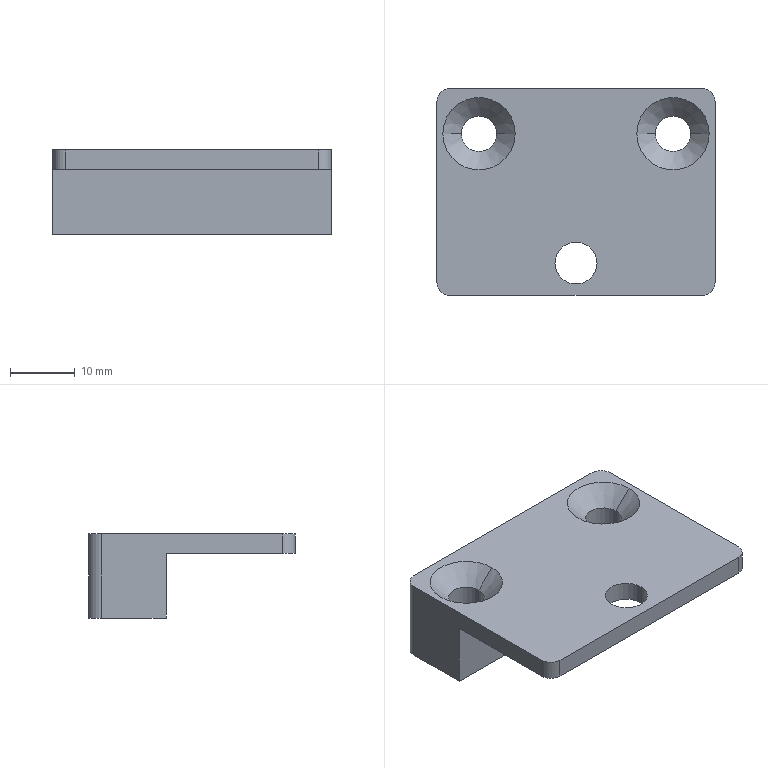Part | SolidWorks | features ICE 2, Extrusion 1, Fillet 1, HoleWzd 1 | 1 solid | 22 faces | box 43 x 32 x 13 mm | volume 8354 mm3 | cylinder 10 | plane 8 | cone 4 | commonest cylinder face diameters 4 x4 5.5 x4 6.5 x2
STEP:
#1=CARTESIAN_POINT('',(18.25,-27.,0.));
#2=VERTEX_POINT('',#1);
#3=CARTESIAN_POINT('',(24.75,-27.,0.));
#4=VERTEX_POINT('',#3);
#5=CARTESIAN_POINT('',(21.5,-27.,0.));
#6=DIRECTION('',(0.,0.,1.));
#7=DIRECTION('',(1.,0.,0.));
#8=AXIS2_PLACEMENT_3D('',#5,#6,#7);
#9=CIRCLE('',#8,3.25);
#10=EDGE_CURVE('',#2,#4,#9,.T.);
#11=ORIENTED_EDGE('',*,*,#10,.F.);
#12=CARTESIAN_POINT('',(18.25,-27.,3.));
#13=VERTEX_POINT('',#12);
#14=CARTESIAN_POINT('',(18.25,-27.,0.));
#15=DIRECTION('',(0.,0.,1.));
#16=VECTOR('',#15,1000.);
#17=LINE('',#14,#16);
#18=EDGE_CURVE('',#2,#13,#17,.T.);
#19=ORIENTED_EDGE('',*,*,#18,.T.);
#20=CARTESIAN_POINT('',(24.75,-27.,3.));
#21=VERTEX_POINT('',#20);
#22=CARTESIAN_POINT('',(21.5,-27.,3.));
#23=DIRECTION('',(0.,0.,1.));
#24=DIRECTION('',(1.,0.,0.));
#25=AXIS2_PLACEMENT_3D('',#22,#23,#24);
#26=CIRCLE('',#25,3.25);
#27=EDGE_CURVE('',#13,#21,#26,.T.);
#28=ORIENTED_EDGE('',*,*,#27,.T.);
#29=CARTESIAN_POINT('',(24.75,-27.,0.));
#30=DIRECTION('',(0.,0.,1.));
#31=VECTOR('',#30,1000.);
#32=LINE('',#29,#31);
#33=EDGE_CURVE('',#4,#21,#32,.T.);
#34=ORIENTED_EDGE('',*,*,#33,.F.);
#35=EDGE_LOOP('',(#11,#19,#28,#34));
#36=FACE_OUTER_BOUND('',#35,.T.);
#37=CARTESIAN_POINT('',(21.5,-27.,0.));
#38=DIRECTION('',(0.,0.,1.));
#39=DIRECTION('',(1.,0.,0.));
#40=AXIS2_PLACEMENT_3D('',#37,#38,#39);
#41=CYLINDRICAL_SURFACE('',#40,3.25);
#42=ADVANCED_FACE('',(#36),#41,.F.);
#43=CARTESIAN_POINT('',(3.75,-7.,0.15));
#44=VERTEX_POINT('',#43);
#45=CARTESIAN_POINT('',(9.25,-7.,0.15));
#46=VERTEX_POINT('',#45);
#47=CARTESIAN_POINT('',(6.5,-7.,0.15));
#48=DIRECTION('',(0.,0.,1.));
#49=DIRECTION('',(1.,0.,0.));
#50=AXIS2_PLACEMENT_3D('',#47,#48,#49);
#51=CIRCLE('',#50,2.75);
#52=EDGE_CURVE('',#44,#46,#51,.T.);
#53=ORIENTED_EDGE('',*,*,#52,.F.);
#54=CARTESIAN_POINT('',(0.9,-7.,3.));
#55=VERTEX_POINT('',#54);
#56=CARTESIAN_POINT('',(0.9,-7.,3.));
#57=DIRECTION('',(-0.7071,0.,0.7071));
#58=VECTOR('',#57,1000.);
#59=LINE('',#56,#58);
#60=EDGE_CURVE('',#44,#55,#59,.T.);
#61=ORIENTED_EDGE('',*,*,#60,.T.);
#62=CARTESIAN_POINT('',(12.1,-7.,3.));
#63=VERTEX_POINT('',#62);
#64=CARTESIAN_POINT('',(6.5,-7.,3.));
#65=DIRECTION('',(0.,0.,1.));
#66=DIRECTION('',(1.,0.,0.));
#67=AXIS2_PLACEMENT_3D('',#64,#65,#66);
#68=CIRCLE('',#67,5.6);
#69=EDGE_CURVE('',#55,#63,#68,.T.);
#70=ORIENTED_EDGE('',*,*,#69,.T.);
#71=CARTESIAN_POINT('',(12.1,-7.,3.));
#72=DIRECTION('',(0.7071,0.,0.7071));
#73=VECTOR('',#72,1000.);
#74=LINE('',#71,#73);
#75=EDGE_CURVE('',#46,#63,#74,.T.);
#76=ORIENTED_EDGE('',*,*,#75,.F.);
#77=EDGE_LOOP('',(#53,#61,#70,#76));
#78=FACE_OUTER_BOUND('',#77,.T.);
#79=CARTESIAN_POINT('',(6.5,-7.,3.));
#80=DIRECTION('',(0.,0.,1.));
#81=DIRECTION('',(1.,0.,0.));
#82=AXIS2_PLACEMENT_3D('',#79,#80,#81);
#83=CONICAL_SURFACE('',#82,5.6,0.7854);
#84=ADVANCED_FACE('',(#78),#83,.F.);
#85=CARTESIAN_POINT('',(3.75,-7.,-10.));
#86=VERTEX_POINT('',#85);
#87=CARTESIAN_POINT('',(9.25,-7.,-10.));
#88=VERTEX_POINT('',#87);
#89=CARTESIAN_POINT('',(6.5,-7.,-10.));
#90=DIRECTION('',(0.,0.,1.));
#91=DIRECTION('',(-1.,0.,0.));
#92=AXIS2_PLACEMENT_3D('',#89,#90,#91);
#93=CIRCLE('',#92,2.75);
#94=EDGE_CURVE('',#86,#88,#93,.T.);
#95=ORIENTED_EDGE('',*,*,#94,.F.);
#96=CARTESIAN_POINT('',(3.75,-7.,3.));
#97=DIRECTION('',(0.,0.,1.));
#98=VECTOR('',#97,1000.);
#99=LINE('',#96,#98);
#100=EDGE_CURVE('',#86,#44,#99,.T.);
#101=ORIENTED_EDGE('',*,*,#100,.T.);
#102=ORIENTED_EDGE('',*,*,#52,.T.);
#103=CARTESIAN_POINT('',(9.25,-7.,3.));
#104=DIRECTION('',(0.,0.,1.));
#105=VECTOR('',#104,1000.);
#106=LINE('',#103,#105);
#107=EDGE_CURVE('',#88,#46,#106,.T.);
#108=ORIENTED_EDGE('',*,*,#107,.F.);
#109=EDGE_LOOP('',(#95,#101,#102,#108));
#110=FACE_OUTER_BOUND('',#109,.T.);
#111=CARTESIAN_POINT('',(6.5,-7.,3.));
#112=DIRECTION('',(0.,0.,1.));
#113=DIRECTION('',(1.,0.,0.));
#114=AXIS2_PLACEMENT_3D('',#111,#112,#113);
#115=CYLINDRICAL_SURFACE('',#114,2.75);
#116=ADVANCED_FACE('',(#110),#115,.F.);
#117=CARTESIAN_POINT('',(33.75,-7.,0.15));
#118=VERTEX_POINT('',#117);
#119=CARTESIAN_POINT('',(39.25,-7.,0.15));
#120=VERTEX_POINT('',#119);
#121=CARTESIAN_POINT('',(36.5,-7.,0.15));
#122=DIRECTION('',(0.,0.,1.));
#123=DIRECTION('',(1.,0.,0.));
#124=AXIS2_PLACEMENT_3D('',#121,#122,#123);
#125=CIRCLE('',#124,2.75);
#126=EDGE_CURVE('',#118,#120,#125,.T.);
#127=ORIENTED_EDGE('',*,*,#126,.F.);
#128=CARTESIAN_POINT('',(30.9,-7.,3.));
#129=VERTEX_POINT('',#128);
#130=CARTESIAN_POINT('',(30.9,-7.,3.));
#131=DIRECTION('',(-0.7071,0.,0.7071));
#132=VECTOR('',#131,1000.);
#133=LINE('',#130,#132);
#134=EDGE_CURVE('',#118,#129,#133,.T.);
#135=ORIENTED_EDGE('',*,*,#134,.T.);
#136=CARTESIAN_POINT('',(42.1,-7.,3.));
#137=VERTEX_POINT('',#136);
#138=CARTESIAN_POINT('',(36.5,-7.,3.));
#139=DIRECTION('',(0.,0.,1.));
#140=DIRECTION('',(1.,0.,0.));
#141=AXIS2_PLACEMENT_3D('',#138,#139,#140);
#142=CIRCLE('',#141,5.6);
#143=EDGE_CURVE('',#129,#137,#142,.T.);
#144=ORIENTED_EDGE('',*,*,#143,.T.);
#145=CARTESIAN_POINT('',(42.1,-7.,3.));
#146=DIRECTION('',(0.7071,0.,0.7071));
#147=VECTOR('',#146,1000.);
#148=LINE('',#145,#147);
#149=EDGE_CURVE('',#120,#137,#148,.T.);
#150=ORIENTED_EDGE('',*,*,#149,.F.);
#151=EDGE_LOOP('',(#127,#135,#144,#150));
#152=FACE_OUTER_BOUND('',#151,.T.);
#153=CARTESIAN_POINT('',(36.5,-7.,3.));
#154=DIRECTION('',(0.,0.,1.));
#155=DIRECTION('',(1.,0.,0.));
#156=AXIS2_PLACEMENT_3D('',#153,#154,#155);
#157=CONICAL_SURFACE('',#156,5.6,0.7854);
#158=ADVANCED_FACE('',(#152),#157,.F.);
#159=CARTESIAN_POINT('',(33.75,-7.,-10.));
#160=VERTEX_POINT('',#159);
#161=CARTESIAN_POINT('',(39.25,-7.,-10.));
#162=VERTEX_POINT('',#161);
#163=CARTESIAN_POINT('',(36.5,-7.,-10.));
#164=DIRECTION('',(0.,0.,1.));
#165=DIRECTION('',(-1.,0.,0.));
#166=AXIS2_PLACEMENT_3D('',#163,#164,#165);
#167=CIRCLE('',#166,2.75);
#168=EDGE_CURVE('',#160,#162,#167,.T.);
#169=ORIENTED_EDGE('',*,*,#168,.F.);
#170=CARTESIAN_POINT('',(33.75,-7.,3.));
#171=DIRECTION('',(0.,0.,1.));
#172=VECTOR('',#171,1000.);
#173=LINE('',#170,#172);
#174=EDGE_CURVE('',#160,#118,#173,.T.);
#175=ORIENTED_EDGE('',*,*,#174,.T.);
#176=ORIENTED_EDGE('',*,*,#126,.T.);
#177=CARTESIAN_POINT('',(39.25,-7.,3.));
#178=DIRECTION('',(0.,0.,1.));
#179=VECTOR('',#178,1000.);
#180=LINE('',#177,#179);
#181=EDGE_CURVE('',#162,#120,#180,.T.);
#182=ORIENTED_EDGE('',*,*,#181,.F.);
#183=EDGE_LOOP('',(#169,#175,#176,#182));
#184=FACE_OUTER_BOUND('',#183,.T.);
#185=CARTESIAN_POINT('',(36.5,-7.,3.));
#186=DIRECTION('',(0.,0.,1.));
#187=DIRECTION('',(1.,0.,0.));
#188=AXIS2_PLACEMENT_3D('',#185,#186,#187);
#189=CYLINDRICAL_SURFACE('',#188,2.75);
#190=ADVANCED_FACE('',(#184),#189,.F.);
#191=CARTESIAN_POINT('',(21.5,-27.,0.));
#192=DIRECTION('',(0.,0.,1.));
#193=DIRECTION('',(1.,0.,0.));
#194=AXIS2_PLACEMENT_3D('',#191,#192,#193);
#195=CIRCLE('',#194,3.25);
#196=EDGE_CURVE('',#4,#2,#195,.T.);
#197=ORIENTED_EDGE('',*,*,#196,.T.);
#198=ORIENTED_EDGE('',*,*,#10,.T.);
#199=EDGE_LOOP('',(#197,#198));
#200=FACE_BOUND('',#199,.T.);
#201=CARTESIAN_POINT('',(43.,-12.,0.));
#202=VERTEX_POINT('',#201);
#203=CARTESIAN_POINT('',(0.,-12.,0.));
#204=VERTEX_POINT('',#203);
#205=CARTESIAN_POINT('',(0.,-12.,0.));
#206=DIRECTION('',(-1.,0.,0.));
#207=VECTOR('',#206,1000.);
#208=LINE('',#205,#207);
#209=EDGE_CURVE('',#202,#204,#208,.T.);
#210=ORIENTED_EDGE('',*,*,#209,.F.);
#211=CARTESIAN_POINT('',(43.,-30.,0.));
#212=VERTEX_POINT('',#211);
#213=CARTESIAN_POINT('',(43.,0.,0.));
#214=DIRECTION('',(0.,1.,0.));
#215=VECTOR('',#214,1000.);
#216=LINE('',#213,#215);
#217=EDGE_CURVE('',#212,#202,#216,.T.);
#218=ORIENTED_EDGE('',*,*,#217,.F.);
#219=CARTESIAN_POINT('',(41.,-32.,0.));
#220=VERTEX_POINT('',#219);
#221=CARTESIAN_POINT('',(41.,-30.,0.));
#222=DIRECTION('',(0.,0.,-1.));
#223=DIRECTION('',(1.,0.,0.));
#224=AXIS2_PLACEMENT_3D('',#221,#222,#223);
#225=CIRCLE('',#224,2.);
#226=EDGE_CURVE('',#212,#220,#225,.T.);
#227=ORIENTED_EDGE('',*,*,#226,.T.);
#228=CARTESIAN_POINT('',(2.,-32.,0.));
#229=VERTEX_POINT('',#228);
#230=CARTESIAN_POINT('',(0.,-32.,0.));
#231=DIRECTION('',(1.,0.,0.));
#232=VECTOR('',#231,1000.);
#233=LINE('',#230,#232);
#234=EDGE_CURVE('',#229,#220,#233,.T.);
#235=ORIENTED_EDGE('',*,*,#234,.F.);
#236=CARTESIAN_POINT('',(0.,-30.,0.));
#237=VERTEX_POINT('',#236);
#238=CARTESIAN_POINT('',(2.,-30.,0.));
#239=DIRECTION('',(0.,0.,-1.));
#240=DIRECTION('',(1.,0.,0.));
#241=AXIS2_PLACEMENT_3D('',#238,#239,#240);
#242=CIRCLE('',#241,2.);
#243=EDGE_CURVE('',#229,#237,#242,.T.);
#244=ORIENTED_EDGE('',*,*,#243,.T.);
#245=CARTESIAN_POINT('',(0.,0.,0.));
#246=DIRECTION('',(0.,-1.,0.));
#247=VECTOR('',#246,1000.);
#248=LINE('',#245,#247);
#249=EDGE_CURVE('',#204,#237,#248,.T.);
#250=ORIENTED_EDGE('',*,*,#249,.F.);
#251=EDGE_LOOP('',(#210,#218,#227,#235,#244,#250));
#252=FACE_OUTER_BOUND('',#251,.T.);
#253=CARTESIAN_POINT('',(0.,0.,0.));
#254=DIRECTION('',(0.,0.,1.));
#255=DIRECTION('',(1.,0.,0.));
#256=AXIS2_PLACEMENT_3D('',#253,#254,#255);
#257=PLANE('',#256);
#258=ADVANCED_FACE('',(#200,#252),#257,.F.);
#259=CARTESIAN_POINT('',(0.,-2.,3.));
#260=VERTEX_POINT('',#259);
#261=CARTESIAN_POINT('',(0.,-30.,3.));
#262=VERTEX_POINT('',#261);
#263=CARTESIAN_POINT('',(0.,0.,3.));
#264=DIRECTION('',(0.,-1.,0.));
#265=VECTOR('',#264,1000.);
#266=LINE('',#263,#265);
#267=EDGE_CURVE('',#260,#262,#266,.T.);
#268=ORIENTED_EDGE('',*,*,#267,.F.);
#269=CARTESIAN_POINT('',(0.,-2.,-10.));
#270=VERTEX_POINT('',#269);
#271=CARTESIAN_POINT('',(0.,-2.,3.));
#272=DIRECTION('',(0.,0.,-1.));
#273=VECTOR('',#272,1000.);
#274=LINE('',#271,#273);
#275=EDGE_CURVE('',#260,#270,#274,.T.);
#276=ORIENTED_EDGE('',*,*,#275,.T.);
#277=CARTESIAN_POINT('',(0.,-12.,-10.));
#278=VERTEX_POINT('',#277);
#279=CARTESIAN_POINT('',(0.,0.,-10.));
#280=DIRECTION('',(0.,1.,0.));
#281=VECTOR('',#280,1000.);
#282=LINE('',#279,#281);
#283=EDGE_CURVE('',#278,#270,#282,.T.);
#284=ORIENTED_EDGE('',*,*,#283,.F.);
#285=CARTESIAN_POINT('',(0.,-12.,-10.));
#286=DIRECTION('',(0.,0.,1.));
#287=VECTOR('',#286,1000.);
#288=LINE('',#285,#287);
#289=EDGE_CURVE('',#278,#204,#288,.T.);
#290=ORIENTED_EDGE('',*,*,#289,.T.);
#291=ORIENTED_EDGE('',*,*,#249,.T.);
#292=CARTESIAN_POINT('',(0.,-30.,3.));
#293=DIRECTION('',(0.,0.,1.));
#294=VECTOR('',#293,1000.);
#295=LINE('',#292,#294);
#296=EDGE_CURVE('',#237,#262,#295,.T.);
#297=ORIENTED_EDGE('',*,*,#296,.T.);
#298=EDGE_LOOP('',(#268,#276,#284,#290,#291,#297));
#299=FACE_OUTER_BOUND('',#298,.T.);
#300=CARTESIAN_POINT('',(0.,0.,3.));
#301=DIRECTION('',(1.,0.,0.));
#302=DIRECTION('',(0.,1.,0.));
#303=AXIS2_PLACEMENT_3D('',#300,#301,#302);
#304=PLANE('',#303);
#305=ADVANCED_FACE('',(#299),#304,.F.);
#306=ORIENTED_EDGE('',*,*,#234,.T.);
#307=CARTESIAN_POINT('',(41.,-32.,3.));
#308=VERTEX_POINT('',#307);
#309=CARTESIAN_POINT('',(41.,-32.,3.));
#310=DIRECTION('',(0.,0.,1.));
#311=VECTOR('',#310,1000.);
#312=LINE('',#309,#311);
#313=EDGE_CURVE('',#220,#308,#312,.T.);
#314=ORIENTED_EDGE('',*,*,#313,.T.);
#315=CARTESIAN_POINT('',(2.,-32.,3.));
#316=VERTEX_POINT('',#315);
#317=CARTESIAN_POINT('',(0.,-32.,3.));
#318=DIRECTION('',(1.,0.,0.));
#319=VECTOR('',#318,1000.);
#320=LINE('',#317,#319);
#321=EDGE_CURVE('',#316,#308,#320,.T.);
#322=ORIENTED_EDGE('',*,*,#321,.F.);
#323=CARTESIAN_POINT('',(2.,-32.,3.));
#324=DIRECTION('',(0.,0.,-1.));
#325=VECTOR('',#324,1000.);
#326=LINE('',#323,#325);
#327=EDGE_CURVE('',#316,#229,#326,.T.);
#328=ORIENTED_EDGE('',*,*,#327,.T.);
#329=EDGE_LOOP('',(#306,#314,#322,#328));
#330=FACE_OUTER_BOUND('',#329,.T.);
#331=CARTESIAN_POINT('',(0.,-32.,3.));
#332=DIRECTION('',(0.,1.,0.));
#333=DIRECTION('',(0.,0.,1.));
#334=AXIS2_PLACEMENT_3D('',#331,#332,#333);
#335=PLANE('',#334);
#336=ADVANCED_FACE('',(#330),#335,.F.);
#337=ORIENTED_EDGE('',*,*,#217,.T.);
#338=CARTESIAN_POINT('',(43.,-12.,-10.));
#339=VERTEX_POINT('',#338);
#340=CARTESIAN_POINT('',(43.,-12.,-10.));
#341=DIRECTION('',(0.,0.,1.));
#342=VECTOR('',#341,1000.);
#343=LINE('',#340,#342);
#344=EDGE_CURVE('',#339,#202,#343,.T.);
#345=ORIENTED_EDGE('',*,*,#344,.F.);
#346=CARTESIAN_POINT('',(43.,-2.,-10.));
#347=VERTEX_POINT('',#346);
#348=CARTESIAN_POINT('',(43.,0.,-10.));
#349=DIRECTION('',(0.,-1.,0.));
#350=VECTOR('',#349,1000.);
#351=LINE('',#348,#350);
#352=EDGE_CURVE('',#347,#339,#351,.T.);
#353=ORIENTED_EDGE('',*,*,#352,.F.);
#354=CARTESIAN_POINT('',(43.,-2.,3.));
#355=VERTEX_POINT('',#354);
#356=CARTESIAN_POINT('',(43.,-2.,3.));
#357=DIRECTION('',(0.,0.,1.));
#358=VECTOR('',#357,1000.);
#359=LINE('',#356,#358);
#360=EDGE_CURVE('',#347,#355,#359,.T.);
#361=ORIENTED_EDGE('',*,*,#360,.T.);
#362=CARTESIAN_POINT('',(43.,-30.,3.));
#363=VERTEX_POINT('',#362);
#364=CARTESIAN_POINT('',(43.,0.,3.));
#365=DIRECTION('',(0.,1.,0.));
#366=VECTOR('',#365,1000.);
#367=LINE('',#364,#366);
#368=EDGE_CURVE('',#363,#355,#367,.T.);
#369=ORIENTED_EDGE('',*,*,#368,.F.);
#370=CARTESIAN_POINT('',(43.,-30.,3.));
#371=DIRECTION('',(0.,0.,-1.));
#372=VECTOR('',#371,1000.);
#373=LINE('',#370,#372);
#374=EDGE_CURVE('',#363,#212,#373,.T.);
#375=ORIENTED_EDGE('',*,*,#374,.T.);
#376=EDGE_LOOP('',(#337,#345,#353,#361,#369,#375));
#377=FACE_OUTER_BOUND('',#376,.T.);
#378=CARTESIAN_POINT('',(43.,0.,3.));
#379=DIRECTION('',(-1.,0.,0.));
#380=DIRECTION('',(0.,-1.,0.));
#381=AXIS2_PLACEMENT_3D('',#378,#379,#380);
#382=PLANE('',#381);
#383=ADVANCED_FACE('',(#377),#382,.F.);
#384=CARTESIAN_POINT('',(41.,0.,3.));
#385=VERTEX_POINT('',#384);
#386=CARTESIAN_POINT('',(2.,0.,3.));
#387=VERTEX_POINT('',#386);
#388=CARTESIAN_POINT('',(0.,0.,3.));
#389=DIRECTION('',(-1.,0.,0.));
#390=VECTOR('',#389,1000.);
#391=LINE('',#388,#390);
#392=EDGE_CURVE('',#385,#387,#391,.T.);
#393=ORIENTED_EDGE('',*,*,#392,.F.);
#394=CARTESIAN_POINT('',(41.,0.,-10.));
#395=VERTEX_POINT('',#394);
#396=CARTESIAN_POINT('',(41.,0.,3.));
#397=DIRECTION('',(0.,0.,-1.));
#398=VECTOR('',#397,1000.);
#399=LINE('',#396,#398);
#400=EDGE_CURVE('',#385,#395,#399,.T.);
#401=ORIENTED_EDGE('',*,*,#400,.T.);
#402=CARTESIAN_POINT('',(2.,0.,-10.));
#403=VERTEX_POINT('',#402);
#404=CARTESIAN_POINT('',(0.,0.,-10.));
#405=DIRECTION('',(1.,0.,0.));
#406=VECTOR('',#405,1000.);
#407=LINE('',#404,#406);
#408=EDGE_CURVE('',#403,#395,#407,.T.);
#409=ORIENTED_EDGE('',*,*,#408,.F.);
#410=CARTESIAN_POINT('',(2.,0.,3.));
#411=DIRECTION('',(0.,0.,1.));
#412=VECTOR('',#411,1000.);
#413=LINE('',#410,#412);
#414=EDGE_CURVE('',#403,#387,#413,.T.);
#415=ORIENTED_EDGE('',*,*,#414,.T.);
#416=EDGE_LOOP('',(#393,#401,#409,#415));
#417=FACE_OUTER_BOUND('',#416,.T.);
#418=CARTESIAN_POINT('',(0.,0.,3.));
#419=DIRECTION('',(0.,-1.,0.));
#420=DIRECTION('',(0.,0.,-1.));
#421=AXIS2_PLACEMENT_3D('',#418,#419,#420);
#422=PLANE('',#421);
#423=ADVANCED_FACE('',(#417),#422,.F.);
#424=CARTESIAN_POINT('',(21.5,-27.,3.));
#425=DIRECTION('',(0.,0.,1.));
#426=DIRECTION('',(1.,0.,0.));
#427=AXIS2_PLACEMENT_3D('',#424,#425,#426);
#428=CIRCLE('',#427,3.25);
#429=EDGE_CURVE('',#21,#13,#428,.T.);
#430=ORIENTED_EDGE('',*,*,#429,.F.);
#431=ORIENTED_EDGE('',*,*,#27,.F.);
#432=EDGE_LOOP('',(#430,#431));
#433=FACE_BOUND('',#432,.T.);
#434=CARTESIAN_POINT('',(6.5,-7.,3.));
#435=DIRECTION('',(0.,0.,1.));
#436=DIRECTION('',(1.,0.,0.));
#437=AXIS2_PLACEMENT_3D('',#434,#435,#436);
#438=CIRCLE('',#437,5.6);
#439=EDGE_CURVE('',#63,#55,#438,.T.);
#440=ORIENTED_EDGE('',*,*,#439,.F.);
#441=ORIENTED_EDGE('',*,*,#69,.F.);
#442=EDGE_LOOP('',(#440,#441));
#443=FACE_BOUND('',#442,.T.);
#444=CARTESIAN_POINT('',(36.5,-7.,3.));
#445=DIRECTION('',(0.,0.,1.));
#446=DIRECTION('',(1.,0.,0.));
#447=AXIS2_PLACEMENT_3D('',#444,#445,#446);
#448=CIRCLE('',#447,5.6);
#449=EDGE_CURVE('',#137,#129,#448,.T.);
#450=ORIENTED_EDGE('',*,*,#449,.F.);
#451=ORIENTED_EDGE('',*,*,#143,.F.);
#452=EDGE_LOOP('',(#450,#451));
#453=FACE_BOUND('',#452,.T.);
#454=ORIENTED_EDGE('',*,*,#368,.T.);
#455=CARTESIAN_POINT('',(41.,-2.,3.));
#456=DIRECTION('',(0.,0.,1.));
#457=DIRECTION('',(1.,0.,0.));
#458=AXIS2_PLACEMENT_3D('',#455,#456,#457);
#459=CIRCLE('',#458,2.);
#460=EDGE_CURVE('',#355,#385,#459,.T.);
#461=ORIENTED_EDGE('',*,*,#460,.T.);
#462=ORIENTED_EDGE('',*,*,#392,.T.);
#463=CARTESIAN_POINT('',(2.,-2.,3.));
#464=DIRECTION('',(0.,0.,1.));
#465=DIRECTION('',(1.,0.,0.));
#466=AXIS2_PLACEMENT_3D('',#463,#464,#465);
#467=CIRCLE('',#466,2.);
#468=EDGE_CURVE('',#387,#260,#467,.T.);
#469=ORIENTED_EDGE('',*,*,#468,.T.);
#470=ORIENTED_EDGE('',*,*,#267,.T.);
#471=CARTESIAN_POINT('',(2.,-30.,3.));
#472=DIRECTION('',(0.,0.,1.));
#473=DIRECTION('',(1.,0.,0.));
#474=AXIS2_PLACEMENT_3D('',#471,#472,#473);
#475=CIRCLE('',#474,2.);
#476=EDGE_CURVE('',#262,#316,#475,.T.);
#477=ORIENTED_EDGE('',*,*,#476,.T.);
#478=ORIENTED_EDGE('',*,*,#321,.T.);
#479=CARTESIAN_POINT('',(41.,-30.,3.));
#480=DIRECTION('',(0.,0.,1.));
#481=DIRECTION('',(1.,0.,0.));
#482=AXIS2_PLACEMENT_3D('',#479,#480,#481);
#483=CIRCLE('',#482,2.);
#484=EDGE_CURVE('',#308,#363,#483,.T.);
#485=ORIENTED_EDGE('',*,*,#484,.T.);
#486=EDGE_LOOP('',(#454,#461,#462,#469,#470,#477,#478,#485));
#487=FACE_OUTER_BOUND('',#486,.T.);
#488=CARTESIAN_POINT('',(0.,0.,3.));
#489=DIRECTION('',(0.,0.,1.));
#490=DIRECTION('',(1.,0.,0.));
#491=AXIS2_PLACEMENT_3D('',#488,#489,#490);
#492=PLANE('',#491);
#493=ADVANCED_FACE('',(#433,#443,#453,#487),#492,.T.);
#494=ORIENTED_EDGE('',*,*,#174,.F.);
#495=CARTESIAN_POINT('',(36.5,-7.,-10.));
#496=DIRECTION('',(0.,0.,1.));
#497=DIRECTION('',(-1.,0.,0.));
#498=AXIS2_PLACEMENT_3D('',#495,#496,#497);
#499=CIRCLE('',#498,2.75);
#500=EDGE_CURVE('',#162,#160,#499,.T.);
#501=ORIENTED_EDGE('',*,*,#500,.F.);
#502=ORIENTED_EDGE('',*,*,#181,.T.);
#503=CARTESIAN_POINT('',(36.5,-7.,0.15));
#504=DIRECTION('',(0.,0.,1.));
#505=DIRECTION('',(1.,0.,0.));
#506=AXIS2_PLACEMENT_3D('',#503,#504,#505);
#507=CIRCLE('',#506,2.75);
#508=EDGE_CURVE('',#120,#118,#507,.T.);
#509=ORIENTED_EDGE('',*,*,#508,.T.);
#510=EDGE_LOOP('',(#494,#501,#502,#509));
#511=FACE_OUTER_BOUND('',#510,.T.);
#512=CARTESIAN_POINT('',(36.5,-7.,3.));
#513=DIRECTION('',(0.,0.,1.));
#514=DIRECTION('',(1.,0.,0.));
#515=AXIS2_PLACEMENT_3D('',#512,#513,#514);
#516=CYLINDRICAL_SURFACE('',#515,2.75);
#517=ADVANCED_FACE('',(#511),#516,.F.);
#518=ORIENTED_EDGE('',*,*,#134,.F.);
#519=ORIENTED_EDGE('',*,*,#508,.F.);
#520=ORIENTED_EDGE('',*,*,#149,.T.);
#521=ORIENTED_EDGE('',*,*,#449,.T.);
#522=EDGE_LOOP('',(#518,#519,#520,#521));
#523=FACE_OUTER_BOUND('',#522,.T.);
#524=CARTESIAN_POINT('',(36.5,-7.,3.));
#525=DIRECTION('',(0.,0.,1.));
#526=DIRECTION('',(1.,0.,0.));
#527=AXIS2_PLACEMENT_3D('',#524,#525,#526);
#528=CONICAL_SURFACE('',#527,5.6,0.7854);
#529=ADVANCED_FACE('',(#523),#528,.F.);
#530=ORIENTED_EDGE('',*,*,#100,.F.);
#531=CARTESIAN_POINT('',(6.5,-7.,-10.));
#532=DIRECTION('',(0.,0.,1.));
#533=DIRECTION('',(-1.,0.,0.));
#534=AXIS2_PLACEMENT_3D('',#531,#532,#533);
#535=CIRCLE('',#534,2.75);
#536=EDGE_CURVE('',#88,#86,#535,.T.);
#537=ORIENTED_EDGE('',*,*,#536,.F.);
#538=ORIENTED_EDGE('',*,*,#107,.T.);
#539=CARTESIAN_POINT('',(6.5,-7.,0.15));
#540=DIRECTION('',(0.,0.,1.));
#541=DIRECTION('',(1.,0.,0.));
#542=AXIS2_PLACEMENT_3D('',#539,#540,#541);
#543=CIRCLE('',#542,2.75);
#544=EDGE_CURVE('',#46,#44,#543,.T.);
#545=ORIENTED_EDGE('',*,*,#544,.T.);
#546=EDGE_LOOP('',(#530,#537,#538,#545));
#547=FACE_OUTER_BOUND('',#546,.T.);
#548=CARTESIAN_POINT('',(6.5,-7.,3.));
#549=DIRECTION('',(0.,0.,1.));
#550=DIRECTION('',(1.,0.,0.));
#551=AXIS2_PLACEMENT_3D('',#548,#549,#550);
#552=CYLINDRICAL_SURFACE('',#551,2.75);
#553=ADVANCED_FACE('',(#547),#552,.F.);
#554=ORIENTED_EDGE('',*,*,#60,.F.);
#555=ORIENTED_EDGE('',*,*,#544,.F.);
#556=ORIENTED_EDGE('',*,*,#75,.T.);
#557=ORIENTED_EDGE('',*,*,#439,.T.);
#558=EDGE_LOOP('',(#554,#555,#556,#557));
#559=FACE_OUTER_BOUND('',#558,.T.);
#560=CARTESIAN_POINT('',(6.5,-7.,3.));
#561=DIRECTION('',(0.,0.,1.));
#562=DIRECTION('',(1.,0.,0.));
#563=AXIS2_PLACEMENT_3D('',#560,#561,#562);
#564=CONICAL_SURFACE('',#563,5.6,0.7854);
#565=ADVANCED_FACE('',(#559),#564,.F.);
#566=ORIENTED_EDGE('',*,*,#18,.F.);
#567=ORIENTED_EDGE('',*,*,#196,.F.);
#568=ORIENTED_EDGE('',*,*,#33,.T.);
#569=ORIENTED_EDGE('',*,*,#429,.T.);
#570=EDGE_LOOP('',(#566,#567,#568,#569));
#571=FACE_OUTER_BOUND('',#570,.T.);
#572=CARTESIAN_POINT('',(21.5,-27.,0.));
#573=DIRECTION('',(0.,0.,1.));
#574=DIRECTION('',(1.,0.,0.));
#575=AXIS2_PLACEMENT_3D('',#572,#573,#574);
#576=CYLINDRICAL_SURFACE('',#575,3.25);
#577=ADVANCED_FACE('',(#571),#576,.F.);
#578=ORIENTED_EDGE('',*,*,#460,.F.);
#579=ORIENTED_EDGE('',*,*,#360,.F.);
#580=CARTESIAN_POINT('',(41.,-2.,-10.));
#581=DIRECTION('',(0.,0.,-1.));
#582=DIRECTION('',(-1.,0.,0.));
#583=AXIS2_PLACEMENT_3D('',#580,#581,#582);
#584=CIRCLE('',#583,2.);
#585=EDGE_CURVE('',#395,#347,#584,.T.);
#586=ORIENTED_EDGE('',*,*,#585,.F.);
#587=ORIENTED_EDGE('',*,*,#400,.F.);
#588=EDGE_LOOP('',(#578,#579,#586,#587));
#589=FACE_OUTER_BOUND('',#588,.T.);
#590=CARTESIAN_POINT('',(41.,-2.,3.));
#591=DIRECTION('',(0.,0.,-1.));
#592=DIRECTION('',(-1.,0.,0.));
#593=AXIS2_PLACEMENT_3D('',#590,#591,#592);
#594=CYLINDRICAL_SURFACE('',#593,2.);
#595=ADVANCED_FACE('',(#589),#594,.T.);
#596=ORIENTED_EDGE('',*,*,#468,.F.);
#597=ORIENTED_EDGE('',*,*,#414,.F.);
#598=CARTESIAN_POINT('',(2.,-2.,-10.));
#599=DIRECTION('',(0.,0.,-1.));
#600=DIRECTION('',(-1.,0.,0.));
#601=AXIS2_PLACEMENT_3D('',#598,#599,#600);
#602=CIRCLE('',#601,2.);
#603=EDGE_CURVE('',#270,#403,#602,.T.);
#604=ORIENTED_EDGE('',*,*,#603,.F.);
#605=ORIENTED_EDGE('',*,*,#275,.F.);
#606=EDGE_LOOP('',(#596,#597,#604,#605));
#607=FACE_OUTER_BOUND('',#606,.T.);
#608=CARTESIAN_POINT('',(2.,-2.,3.));
#609=DIRECTION('',(0.,0.,-1.));
#610=DIRECTION('',(-1.,0.,0.));
#611=AXIS2_PLACEMENT_3D('',#608,#609,#610);
#612=CYLINDRICAL_SURFACE('',#611,2.);
#613=ADVANCED_FACE('',(#607),#612,.T.);
#614=ORIENTED_EDGE('',*,*,#484,.F.);
#615=ORIENTED_EDGE('',*,*,#313,.F.);
#616=ORIENTED_EDGE('',*,*,#226,.F.);
#617=ORIENTED_EDGE('',*,*,#374,.F.);
#618=EDGE_LOOP('',(#614,#615,#616,#617));
#619=FACE_OUTER_BOUND('',#618,.T.);
#620=CARTESIAN_POINT('',(41.,-30.,3.));
#621=DIRECTION('',(0.,0.,-1.));
#622=DIRECTION('',(-1.,0.,0.));
#623=AXIS2_PLACEMENT_3D('',#620,#621,#622);
#624=CYLINDRICAL_SURFACE('',#623,2.);
#625=ADVANCED_FACE('',(#619),#624,.T.);
#626=ORIENTED_EDGE('',*,*,#476,.F.);
#627=ORIENTED_EDGE('',*,*,#296,.F.);
#628=ORIENTED_EDGE('',*,*,#243,.F.);
#629=ORIENTED_EDGE('',*,*,#327,.F.);
#630=EDGE_LOOP('',(#626,#627,#628,#629));
#631=FACE_OUTER_BOUND('',#630,.T.);
#632=CARTESIAN_POINT('',(2.,-30.,3.));
#633=DIRECTION('',(0.,0.,-1.));
#634=DIRECTION('',(-1.,0.,0.));
#635=AXIS2_PLACEMENT_3D('',#632,#633,#634);
#636=CYLINDRICAL_SURFACE('',#635,2.);
#637=ADVANCED_FACE('',(#631),#636,.T.);
#638=ORIENTED_EDGE('',*,*,#209,.T.);
#639=ORIENTED_EDGE('',*,*,#289,.F.);
#640=CARTESIAN_POINT('',(0.,-12.,-10.));
#641=DIRECTION('',(-1.,0.,0.));
#642=VECTOR('',#641,1000.);
#643=LINE('',#640,#642);
#644=EDGE_CURVE('',#339,#278,#643,.T.);
#645=ORIENTED_EDGE('',*,*,#644,.F.);
#646=ORIENTED_EDGE('',*,*,#344,.T.);
#647=EDGE_LOOP('',(#638,#639,#645,#646));
#648=FACE_OUTER_BOUND('',#647,.T.);
#649=CARTESIAN_POINT('',(0.,-12.,-10.));
#650=DIRECTION('',(0.,1.,0.));
#651=DIRECTION('',(-1.,0.,0.));
#652=AXIS2_PLACEMENT_3D('',#649,#650,#651);
#653=PLANE('',#652);
#654=ADVANCED_FACE('',(#648),#653,.F.);
#655=ORIENTED_EDGE('',*,*,#500,.T.);
#656=ORIENTED_EDGE('',*,*,#168,.T.);
#657=EDGE_LOOP('',(#655,#656));
#658=FACE_BOUND('',#657,.T.);
#659=ORIENTED_EDGE('',*,*,#536,.T.);
#660=ORIENTED_EDGE('',*,*,#94,.T.);
#661=EDGE_LOOP('',(#659,#660));
#662=FACE_BOUND('',#661,.T.);
#663=ORIENTED_EDGE('',*,*,#352,.T.);
#664=ORIENTED_EDGE('',*,*,#644,.T.);
#665=ORIENTED_EDGE('',*,*,#283,.T.);
#666=ORIENTED_EDGE('',*,*,#603,.T.);
#667=ORIENTED_EDGE('',*,*,#408,.T.);
#668=ORIENTED_EDGE('',*,*,#585,.T.);
#669=EDGE_LOOP('',(#663,#664,#665,#666,#667,#668));
#670=FACE_OUTER_BOUND('',#669,.T.);
#671=CARTESIAN_POINT('',(0.,0.,-10.));
#672=DIRECTION('',(0.,0.,-1.));
#673=DIRECTION('',(-1.,0.,0.));
#674=AXIS2_PLACEMENT_3D('',#671,#672,#673);
#675=PLANE('',#674);
#676=ADVANCED_FACE('',(#658,#662,#670),#675,.T.);
#677=CLOSED_SHELL('',(#42,#84,#116,#158,#190,#258,#305,#336,#383,#423,#493,#517,#529,#553,#565,#577,#595,#613,#625,#637,#654,#676));
#678=MANIFOLD_SOLID_BREP('',#677);
#679=CARTESIAN_POINT('',(0.,0.,0.));
#680=DIRECTION('',(0.,0.,1.));
#681=DIRECTION('',(1.,0.,0.));
#682=AXIS2_PLACEMENT_3D('',#679,#680,#681);
#683=(LENGTH_UNIT()NAMED_UNIT(*)SI_UNIT(.MILLI.,.METRE.));
#684=UNCERTAINTY_MEASURE_WITH_UNIT(LENGTH_MEASURE(0.00001),#683,'','');
#685=(NAMED_UNIT(*)PLANE_ANGLE_UNIT()SI_UNIT($,.RADIAN.));
#686=(NAMED_UNIT(*)SI_UNIT($,.STERADIAN.)SOLID_ANGLE_UNIT());
#687=(GEOMETRIC_REPRESENTATION_CONTEXT(3)GLOBAL_UNCERTAINTY_ASSIGNED_CONTEXT((#684))GLOBAL_UNIT_ASSIGNED_CONTEXT((#683,#685,#686))REPRESENTATION_CONTEXT('',''));
#688=ADVANCED_BREP_SHAPE_REPRESENTATION('',(#678,#682),#687);